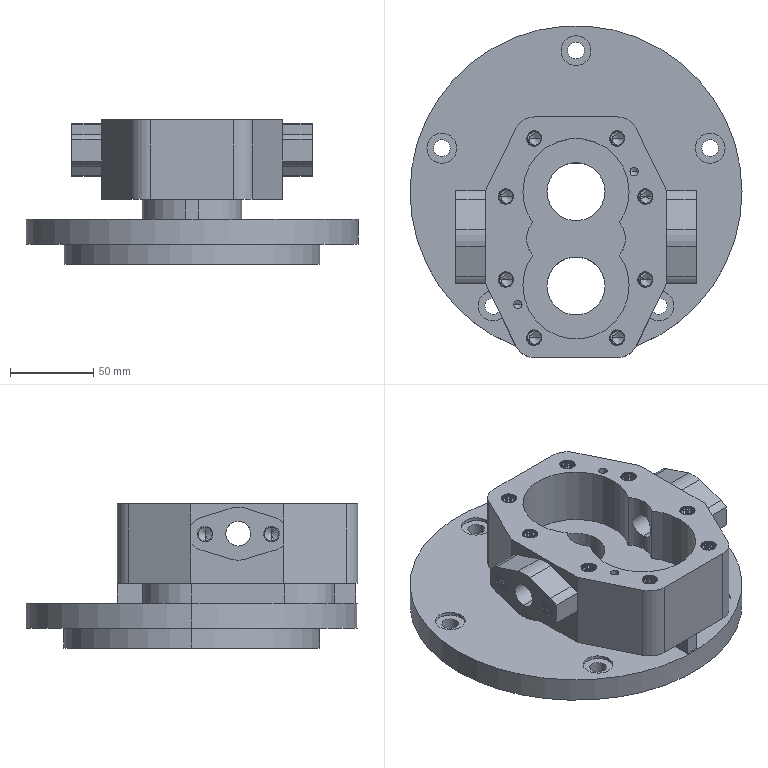Part | SolidWorks | features SweepThread 12, ICE 11, HoleWzd 3, MirrorPattern 2, Rib 2, 3DProfileFeature 1, Extrusion 1 | 1 solid | 702 faces | box 200 x 200 x 87 mm | volume 962197 mm3 | cylinder 553 | plane 57 | cone 56 | spline 36 | commonest cylinder face diameters 8.5 x476 10 x10 18 x10 20 x8 45 x6 64 x6